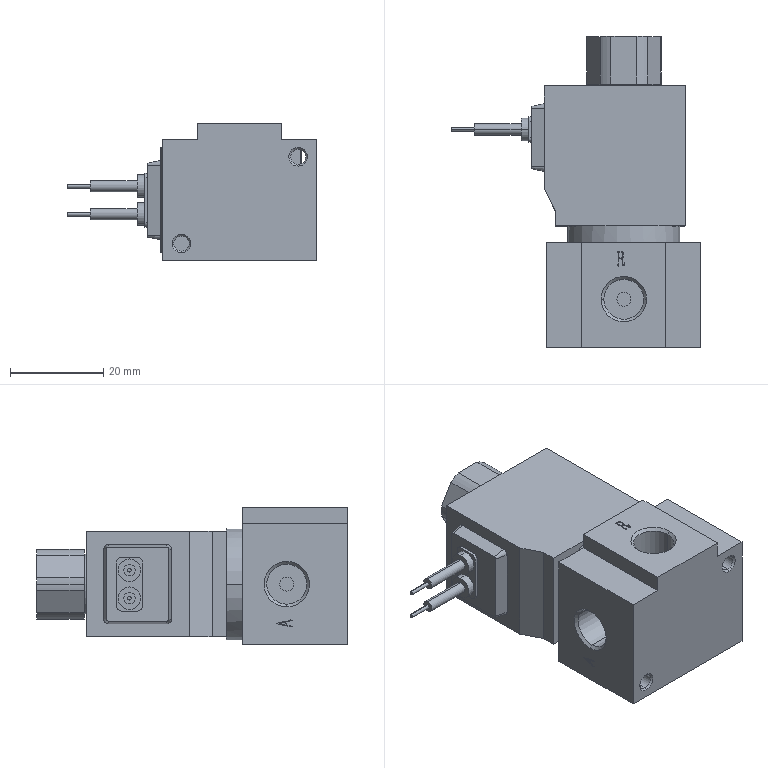Part | 1 solid | 209 faces | box 53.5 x 66.6 x 29.5 mm | volume 43067 mm3 | plane 109 | cylinder 52 | spline 34 | cone 14 | commonest cylinder face diameters 16 x7 3 x6 8.566 x6 0.8 x4 2 x4 2.4 x4